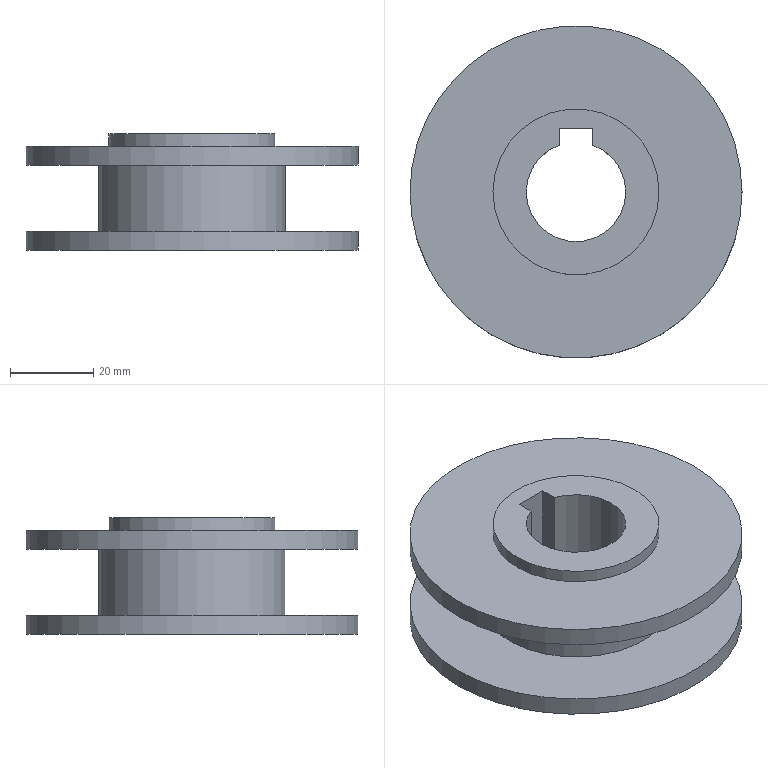Part | NX | features EXTRUDE 3, DATUM_CSYS 1, LINKED_FACE 1, SKETCH 1, UNITE 1 | 1 solid | 13 faces | box 80 x 80 x 28 mm | volume 60999 mm3 | plane 8 | cylinder 5 | commonest cylinder face diameters 80 x2 24 x1 40 x1 45 x1
STEP:
#1=CARTESIAN_POINT('',(40.,0.,12.5));
#2=VERTEX_POINT('',#1);
#3=CARTESIAN_POINT('',(0.,0.,12.5));
#4=DIRECTION('',(0.,0.,1.));
#5=DIRECTION('',(1.,0.,0.));
#6=AXIS2_PLACEMENT_3D('',#3,#4,#5);
#7=CIRCLE('',#6,40.);
#8=EDGE_CURVE('',#2,#2,#7,.T.);
#9=ORIENTED_EDGE('',*,*,#8,.F.);
#10=EDGE_LOOP('',(#9));
#11=FACE_BOUND('',#10,.T.);
#12=CARTESIAN_POINT('',(40.,0.,8.));
#13=VERTEX_POINT('',#12);
#14=CARTESIAN_POINT('',(0.,0.,8.));
#15=DIRECTION('',(0.,0.,1.));
#16=DIRECTION('',(1.,0.,0.));
#17=AXIS2_PLACEMENT_3D('',#14,#15,#16);
#18=CIRCLE('',#17,40.);
#19=EDGE_CURVE('',#13,#13,#18,.T.);
#20=ORIENTED_EDGE('',*,*,#19,.T.);
#21=EDGE_LOOP('',(#20));
#22=FACE_BOUND('',#21,.T.);
#23=CARTESIAN_POINT('',(0.,0.,-12.5));
#24=DIRECTION('',(0.,0.,1.));
#25=DIRECTION('',(1.,0.,0.));
#26=AXIS2_PLACEMENT_3D('',#23,#24,#25);
#27=CYLINDRICAL_SURFACE('',#26,40.);
#28=ADVANCED_FACE('',(#11,#22),#27,.T.);
#29=CARTESIAN_POINT('',(-4.,15.3,-12.5));
#30=VERTEX_POINT('',#29);
#31=CARTESIAN_POINT('',(-4.,15.3,15.5));
#32=VERTEX_POINT('',#31);
#33=CARTESIAN_POINT('',(-4.,15.3,-12.5));
#34=DIRECTION('',(0.,0.,1.));
#35=VECTOR('',#34,1000.);
#36=LINE('',#33,#35);
#37=EDGE_CURVE('',#30,#32,#36,.T.);
#38=ORIENTED_EDGE('',*,*,#37,.T.);
#39=CARTESIAN_POINT('',(-4.,11.314,15.5));
#40=VERTEX_POINT('',#39);
#41=CARTESIAN_POINT('',(-4.,11.314,15.5));
#42=DIRECTION('',(0.,1.,0.));
#43=VECTOR('',#42,1000.);
#44=LINE('',#41,#43);
#45=EDGE_CURVE('',#40,#32,#44,.T.);
#46=ORIENTED_EDGE('',*,*,#45,.F.);
#47=CARTESIAN_POINT('',(-4.,11.314,-12.5));
#48=VERTEX_POINT('',#47);
#49=CARTESIAN_POINT('',(-4.,11.314,-12.5));
#50=DIRECTION('',(0.,0.,1.));
#51=VECTOR('',#50,1000.);
#52=LINE('',#49,#51);
#53=EDGE_CURVE('',#48,#40,#52,.T.);
#54=ORIENTED_EDGE('',*,*,#53,.F.);
#55=CARTESIAN_POINT('',(-4.,11.314,-12.5));
#56=DIRECTION('',(0.,1.,0.));
#57=VECTOR('',#56,1000.);
#58=LINE('',#55,#57);
#59=EDGE_CURVE('',#48,#30,#58,.T.);
#60=ORIENTED_EDGE('',*,*,#59,.T.);
#61=EDGE_LOOP('',(#38,#46,#54,#60));
#62=FACE_BOUND('',#61,.T.);
#63=CARTESIAN_POINT('',(-4.,11.314,-12.5));
#64=DIRECTION('',(1.,0.,0.));
#65=DIRECTION('',(0.,0.,-1.));
#66=AXIS2_PLACEMENT_3D('',#63,#64,#65);
#67=PLANE('',#66);
#68=ADVANCED_FACE('',(#62),#67,.T.);
#69=CARTESIAN_POINT('',(4.,15.3,-12.5));
#70=VERTEX_POINT('',#69);
#71=CARTESIAN_POINT('',(4.,15.3,15.5));
#72=VERTEX_POINT('',#71);
#73=CARTESIAN_POINT('',(4.,15.3,-12.5));
#74=DIRECTION('',(0.,0.,1.));
#75=VECTOR('',#74,1000.);
#76=LINE('',#73,#75);
#77=EDGE_CURVE('',#70,#72,#76,.T.);
#78=ORIENTED_EDGE('',*,*,#77,.T.);
#79=CARTESIAN_POINT('',(-4.,15.3,15.5));
#80=DIRECTION('',(1.,0.,0.));
#81=VECTOR('',#80,1000.);
#82=LINE('',#79,#81);
#83=EDGE_CURVE('',#32,#72,#82,.T.);
#84=ORIENTED_EDGE('',*,*,#83,.F.);
#85=ORIENTED_EDGE('',*,*,#37,.F.);
#86=CARTESIAN_POINT('',(-4.,15.3,-12.5));
#87=DIRECTION('',(1.,0.,0.));
#88=VECTOR('',#87,1000.);
#89=LINE('',#86,#88);
#90=EDGE_CURVE('',#30,#70,#89,.T.);
#91=ORIENTED_EDGE('',*,*,#90,.T.);
#92=EDGE_LOOP('',(#78,#84,#85,#91));
#93=FACE_BOUND('',#92,.T.);
#94=CARTESIAN_POINT('',(-4.,15.3,-12.5));
#95=DIRECTION('',(0.,-1.,0.));
#96=DIRECTION('',(0.,0.,-1.));
#97=AXIS2_PLACEMENT_3D('',#94,#95,#96);
#98=PLANE('',#97);
#99=ADVANCED_FACE('',(#93),#98,.T.);
#100=CARTESIAN_POINT('',(4.,11.314,-12.5));
#101=VERTEX_POINT('',#100);
#102=CARTESIAN_POINT('',(4.,11.314,15.5));
#103=VERTEX_POINT('',#102);
#104=CARTESIAN_POINT('',(4.,11.314,-12.5));
#105=DIRECTION('',(0.,0.,1.));
#106=VECTOR('',#105,1000.);
#107=LINE('',#104,#106);
#108=EDGE_CURVE('',#101,#103,#107,.T.);
#109=ORIENTED_EDGE('',*,*,#108,.T.);
#110=CARTESIAN_POINT('',(4.,15.3,15.5));
#111=DIRECTION('',(0.,-1.,0.));
#112=VECTOR('',#111,1000.);
#113=LINE('',#110,#112);
#114=EDGE_CURVE('',#72,#103,#113,.T.);
#115=ORIENTED_EDGE('',*,*,#114,.F.);
#116=ORIENTED_EDGE('',*,*,#77,.F.);
#117=CARTESIAN_POINT('',(4.,15.3,-12.5));
#118=DIRECTION('',(0.,-1.,0.));
#119=VECTOR('',#118,1000.);
#120=LINE('',#117,#119);
#121=EDGE_CURVE('',#70,#101,#120,.T.);
#122=ORIENTED_EDGE('',*,*,#121,.T.);
#123=EDGE_LOOP('',(#109,#115,#116,#122));
#124=FACE_BOUND('',#123,.T.);
#125=CARTESIAN_POINT('',(4.,15.3,-12.5));
#126=DIRECTION('',(-1.,0.,0.));
#127=DIRECTION('',(0.,0.,1.));
#128=AXIS2_PLACEMENT_3D('',#125,#126,#127);
#129=PLANE('',#128);
#130=ADVANCED_FACE('',(#124),#129,.T.);
#131=CARTESIAN_POINT('',(-40.,0.,-8.));
#132=VERTEX_POINT('',#131);
#133=CARTESIAN_POINT('',(0.,0.,-8.));
#134=DIRECTION('',(0.,0.,1.));
#135=DIRECTION('',(-1.,0.,0.));
#136=AXIS2_PLACEMENT_3D('',#133,#134,#135);
#137=CIRCLE('',#136,40.);
#138=EDGE_CURVE('',#132,#132,#137,.T.);
#139=ORIENTED_EDGE('',*,*,#138,.F.);
#140=EDGE_LOOP('',(#139));
#141=FACE_BOUND('',#140,.T.);
#142=CARTESIAN_POINT('',(-40.,0.,-12.5));
#143=VERTEX_POINT('',#142);
#144=CARTESIAN_POINT('',(0.,0.,-12.5));
#145=DIRECTION('',(0.,0.,1.));
#146=DIRECTION('',(-1.,0.,0.));
#147=AXIS2_PLACEMENT_3D('',#144,#145,#146);
#148=CIRCLE('',#147,40.);
#149=EDGE_CURVE('',#143,#143,#148,.T.);
#150=ORIENTED_EDGE('',*,*,#149,.T.);
#151=EDGE_LOOP('',(#150));
#152=FACE_BOUND('',#151,.T.);
#153=CARTESIAN_POINT('',(0.,0.,-12.5));
#154=DIRECTION('',(0.,0.,1.));
#155=DIRECTION('',(1.,0.,0.));
#156=AXIS2_PLACEMENT_3D('',#153,#154,#155);
#157=CYLINDRICAL_SURFACE('',#156,40.);
#158=ADVANCED_FACE('',(#141,#152),#157,.T.);
#159=ORIENTED_EDGE('',*,*,#53,.T.);
#160=CARTESIAN_POINT('',(0.,0.,15.5));
#161=DIRECTION('',(0.,0.,-1.));
#162=DIRECTION('',(0.3333,0.9428,0.));
#163=AXIS2_PLACEMENT_3D('',#160,#161,#162);
#164=CIRCLE('',#163,12.);
#165=EDGE_CURVE('',#103,#40,#164,.T.);
#166=ORIENTED_EDGE('',*,*,#165,.F.);
#167=ORIENTED_EDGE('',*,*,#108,.F.);
#168=CARTESIAN_POINT('',(0.,0.,-12.5));
#169=DIRECTION('',(0.,0.,-1.));
#170=DIRECTION('',(0.3333,0.9428,0.));
#171=AXIS2_PLACEMENT_3D('',#168,#169,#170);
#172=CIRCLE('',#171,12.);
#173=EDGE_CURVE('',#101,#48,#172,.T.);
#174=ORIENTED_EDGE('',*,*,#173,.T.);
#175=EDGE_LOOP('',(#159,#166,#167,#174));
#176=FACE_BOUND('',#175,.T.);
#177=CARTESIAN_POINT('',(0.,0.,-12.5));
#178=DIRECTION('',(0.,0.,1.));
#179=DIRECTION('',(1.,0.,0.));
#180=AXIS2_PLACEMENT_3D('',#177,#178,#179);
#181=CYLINDRICAL_SURFACE('',#180,12.);
#182=ADVANCED_FACE('',(#176),#181,.F.);
#183=ORIENTED_EDGE('',*,*,#149,.F.);
#184=EDGE_LOOP('',(#183));
#185=FACE_BOUND('',#184,.T.);
#186=ORIENTED_EDGE('',*,*,#59,.F.);
#187=ORIENTED_EDGE('',*,*,#173,.F.);
#188=ORIENTED_EDGE('',*,*,#121,.F.);
#189=ORIENTED_EDGE('',*,*,#90,.F.);
#190=EDGE_LOOP('',(#186,#187,#188,#189));
#191=FACE_BOUND('',#190,.T.);
#192=CARTESIAN_POINT('',(0.,0.,-12.5));
#193=DIRECTION('',(0.,0.,1.));
#194=DIRECTION('',(1.,0.,0.));
#195=AXIS2_PLACEMENT_3D('',#192,#193,#194);
#196=PLANE('',#195);
#197=ADVANCED_FACE('',(#185,#191),#196,.F.);
#198=CARTESIAN_POINT('',(20.,0.,12.5));
#199=VERTEX_POINT('',#198);
#200=CARTESIAN_POINT('',(0.,0.,12.5));
#201=DIRECTION('',(0.,0.,1.));
#202=DIRECTION('',(1.,0.,0.));
#203=AXIS2_PLACEMENT_3D('',#200,#201,#202);
#204=CIRCLE('',#203,20.);
#205=EDGE_CURVE('',#199,#199,#204,.T.);
#206=ORIENTED_EDGE('',*,*,#205,.F.);
#207=EDGE_LOOP('',(#206));
#208=FACE_BOUND('',#207,.T.);
#209=ORIENTED_EDGE('',*,*,#8,.T.);
#210=EDGE_LOOP('',(#209));
#211=FACE_BOUND('',#210,.T.);
#212=CARTESIAN_POINT('',(0.,0.,12.5));
#213=DIRECTION('',(0.,0.,1.));
#214=DIRECTION('',(1.,0.,0.));
#215=AXIS2_PLACEMENT_3D('',#212,#213,#214);
#216=PLANE('',#215);
#217=ADVANCED_FACE('',(#208,#211),#216,.T.);
#218=CARTESIAN_POINT('',(0.,22.5,8.));
#219=VERTEX_POINT('',#218);
#220=CARTESIAN_POINT('',(0.,0.,8.));
#221=DIRECTION('',(0.,0.,-1.));
#222=DIRECTION('',(0.,1.,0.));
#223=AXIS2_PLACEMENT_3D('',#220,#221,#222);
#224=CIRCLE('',#223,22.5);
#225=EDGE_CURVE('',#219,#219,#224,.F.);
#226=ORIENTED_EDGE('',*,*,#225,.F.);
#227=EDGE_LOOP('',(#226));
#228=FACE_BOUND('',#227,.T.);
#229=CARTESIAN_POINT('',(0.,22.5,-8.));
#230=VERTEX_POINT('',#229);
#231=CARTESIAN_POINT('',(0.,0.,-8.));
#232=DIRECTION('',(0.,0.,-1.));
#233=DIRECTION('',(0.,1.,0.));
#234=AXIS2_PLACEMENT_3D('',#231,#232,#233);
#235=CIRCLE('',#234,22.5);
#236=EDGE_CURVE('',#230,#230,#235,.F.);
#237=ORIENTED_EDGE('',*,*,#236,.T.);
#238=EDGE_LOOP('',(#237));
#239=FACE_BOUND('',#238,.T.);
#240=CARTESIAN_POINT('',(0.,0.,-8.));
#241=DIRECTION('',(0.,0.,1.));
#242=DIRECTION('',(1.,0.,0.));
#243=AXIS2_PLACEMENT_3D('',#240,#241,#242);
#244=CYLINDRICAL_SURFACE('',#243,22.5);
#245=ADVANCED_FACE('',(#228,#239),#244,.T.);
#246=ORIENTED_EDGE('',*,*,#138,.T.);
#247=EDGE_LOOP('',(#246));
#248=FACE_BOUND('',#247,.T.);
#249=ORIENTED_EDGE('',*,*,#236,.F.);
#250=EDGE_LOOP('',(#249));
#251=FACE_BOUND('',#250,.T.);
#252=CARTESIAN_POINT('',(0.,0.,-8.));
#253=DIRECTION('',(0.,0.,1.));
#254=DIRECTION('',(1.,0.,0.));
#255=AXIS2_PLACEMENT_3D('',#252,#253,#254);
#256=PLANE('',#255);
#257=ADVANCED_FACE('',(#248,#251),#256,.T.);
#258=ORIENTED_EDGE('',*,*,#19,.F.);
#259=EDGE_LOOP('',(#258));
#260=FACE_BOUND('',#259,.T.);
#261=ORIENTED_EDGE('',*,*,#225,.T.);
#262=EDGE_LOOP('',(#261));
#263=FACE_BOUND('',#262,.T.);
#264=CARTESIAN_POINT('',(0.,0.,8.));
#265=DIRECTION('',(0.,0.,1.));
#266=DIRECTION('',(1.,0.,0.));
#267=AXIS2_PLACEMENT_3D('',#264,#265,#266);
#268=PLANE('',#267);
#269=ADVANCED_FACE('',(#260,#263),#268,.F.);
#270=ORIENTED_EDGE('',*,*,#205,.T.);
#271=EDGE_LOOP('',(#270));
#272=FACE_BOUND('',#271,.T.);
#273=CARTESIAN_POINT('',(-20.,0.,15.5));
#274=VERTEX_POINT('',#273);
#275=CARTESIAN_POINT('',(0.,0.,15.5));
#276=DIRECTION('',(0.,0.,1.));
#277=DIRECTION('',(-1.,0.,0.));
#278=AXIS2_PLACEMENT_3D('',#275,#276,#277);
#279=CIRCLE('',#278,20.);
#280=EDGE_CURVE('',#274,#274,#279,.T.);
#281=ORIENTED_EDGE('',*,*,#280,.F.);
#282=EDGE_LOOP('',(#281));
#283=FACE_BOUND('',#282,.T.);
#284=CARTESIAN_POINT('',(0.,0.,15.5));
#285=DIRECTION('',(0.,0.,-1.));
#286=DIRECTION('',(-1.,0.,0.));
#287=AXIS2_PLACEMENT_3D('',#284,#285,#286);
#288=CYLINDRICAL_SURFACE('',#287,20.);
#289=ADVANCED_FACE('',(#272,#283),#288,.T.);
#290=ORIENTED_EDGE('',*,*,#280,.T.);
#291=EDGE_LOOP('',(#290));
#292=FACE_BOUND('',#291,.T.);
#293=ORIENTED_EDGE('',*,*,#45,.T.);
#294=ORIENTED_EDGE('',*,*,#83,.T.);
#295=ORIENTED_EDGE('',*,*,#114,.T.);
#296=ORIENTED_EDGE('',*,*,#165,.T.);
#297=EDGE_LOOP('',(#293,#294,#295,#296));
#298=FACE_BOUND('',#297,.T.);
#299=CARTESIAN_POINT('',(0.,0.,15.5));
#300=DIRECTION('',(0.,0.,1.));
#301=DIRECTION('',(1.,0.,0.));
#302=AXIS2_PLACEMENT_3D('',#299,#300,#301);
#303=PLANE('',#302);
#304=ADVANCED_FACE('',(#292,#298),#303,.T.);
#305=CLOSED_SHELL('',(#28,#68,#99,#130,#158,#182,#197,#217,#245,#257,#269,#289,#304));
#306=MANIFOLD_SOLID_BREP('',#305);
#307=(LENGTH_UNIT()NAMED_UNIT(*)SI_UNIT(.MILLI.,.METRE.));
#308=UNCERTAINTY_MEASURE_WITH_UNIT(LENGTH_MEASURE(0.00001),#307,'','');
#309=(NAMED_UNIT(*)PLANE_ANGLE_UNIT()SI_UNIT($,.RADIAN.));
#310=(NAMED_UNIT(*)SI_UNIT($,.STERADIAN.)SOLID_ANGLE_UNIT());
#311=(GEOMETRIC_REPRESENTATION_CONTEXT(3)GLOBAL_UNCERTAINTY_ASSIGNED_CONTEXT((#308))GLOBAL_UNIT_ASSIGNED_CONTEXT((#307,#309,#310))REPRESENTATION_CONTEXT('',''));
#312=ADVANCED_BREP_SHAPE_REPRESENTATION('',(#306),#311);